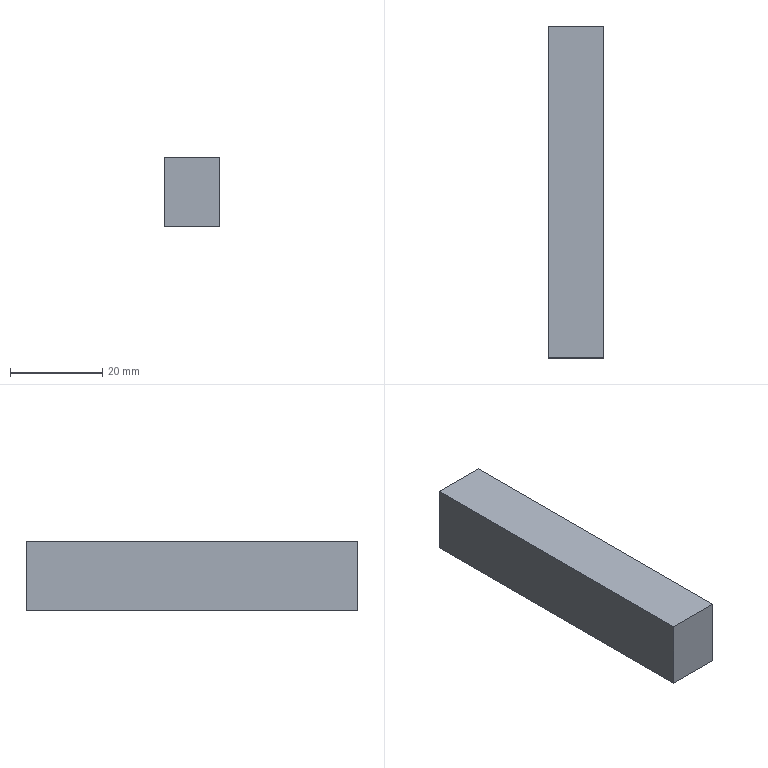Part | NX | features solid 2 | 1 solid | 6 faces | box 12 x 72 x 15 mm | volume 12960 mm3 | plane 6
STEP:
#1=CARTESIAN_POINT('',(546.,577.,-10.));
#2=VERTEX_POINT('',#1);
#3=CARTESIAN_POINT('',(558.,577.,-10.));
#4=VERTEX_POINT('',#3);
#5=CARTESIAN_POINT('',(582.,577.,-10.));
#6=DIRECTION('',(-1.,0.,0.));
#7=VECTOR('',#6,1000.);
#8=LINE('',#5,#7);
#9=EDGE_CURVE('',#2,#4,#8,.F.);
#10=ORIENTED_EDGE('',*,*,#9,.F.);
#11=CARTESIAN_POINT('',(546.,577.,-25.));
#12=VERTEX_POINT('',#11);
#13=CARTESIAN_POINT('',(546.,577.,84.523));
#14=DIRECTION('',(0.,0.,-1.));
#15=VECTOR('',#14,1000.);
#16=LINE('',#13,#15);
#17=EDGE_CURVE('',#2,#12,#16,.T.);
#18=ORIENTED_EDGE('',*,*,#17,.T.);
#19=CARTESIAN_POINT('',(558.,577.,-25.));
#20=VERTEX_POINT('',#19);
#21=CARTESIAN_POINT('',(525.,577.,-25.));
#22=DIRECTION('',(1.,0.,0.));
#23=VECTOR('',#22,1000.);
#24=LINE('',#21,#23);
#25=EDGE_CURVE('',#12,#20,#24,.T.);
#26=ORIENTED_EDGE('',*,*,#25,.T.);
#27=CARTESIAN_POINT('',(558.,577.,84.523));
#28=DIRECTION('',(0.,0.,-1.));
#29=VECTOR('',#28,1000.);
#30=LINE('',#27,#29);
#31=EDGE_CURVE('',#4,#20,#30,.T.);
#32=ORIENTED_EDGE('',*,*,#31,.F.);
#33=EDGE_LOOP('',(#10,#18,#26,#32));
#34=FACE_BOUND('',#33,.T.);
#35=CARTESIAN_POINT('',(546.,577.,-10.));
#36=DIRECTION('',(0.,-1.,0.));
#37=DIRECTION('',(0.,0.,-1.));
#38=AXIS2_PLACEMENT_3D('',#35,#36,#37);
#39=PLANE('',#38);
#40=ADVANCED_FACE('',(#34),#39,.T.);
#41=CARTESIAN_POINT('',(546.,649.,-10.));
#42=VERTEX_POINT('',#41);
#43=CARTESIAN_POINT('',(546.,649.,-25.));
#44=VERTEX_POINT('',#43);
#45=CARTESIAN_POINT('',(546.,649.,84.523));
#46=DIRECTION('',(0.,0.,-1.));
#47=VECTOR('',#46,1000.);
#48=LINE('',#45,#47);
#49=EDGE_CURVE('',#42,#44,#48,.T.);
#50=ORIENTED_EDGE('',*,*,#49,.F.);
#51=CARTESIAN_POINT('',(558.,649.,-10.));
#52=VERTEX_POINT('',#51);
#53=CARTESIAN_POINT('',(525.,649.,-10.));
#54=DIRECTION('',(1.,0.,0.));
#55=VECTOR('',#54,1000.);
#56=LINE('',#53,#55);
#57=EDGE_CURVE('',#42,#52,#56,.T.);
#58=ORIENTED_EDGE('',*,*,#57,.T.);
#59=CARTESIAN_POINT('',(558.,649.,-25.));
#60=VERTEX_POINT('',#59);
#61=CARTESIAN_POINT('',(558.,649.,84.523));
#62=DIRECTION('',(0.,0.,-1.));
#63=VECTOR('',#62,1000.);
#64=LINE('',#61,#63);
#65=EDGE_CURVE('',#52,#60,#64,.T.);
#66=ORIENTED_EDGE('',*,*,#65,.T.);
#67=CARTESIAN_POINT('',(525.,649.,-25.));
#68=DIRECTION('',(1.,0.,0.));
#69=VECTOR('',#68,1000.);
#70=LINE('',#67,#69);
#71=EDGE_CURVE('',#44,#60,#70,.T.);
#72=ORIENTED_EDGE('',*,*,#71,.F.);
#73=EDGE_LOOP('',(#50,#58,#66,#72));
#74=FACE_BOUND('',#73,.T.);
#75=CARTESIAN_POINT('',(546.,649.,-10.));
#76=DIRECTION('',(0.,-1.,0.));
#77=DIRECTION('',(0.,0.,-1.));
#78=AXIS2_PLACEMENT_3D('',#75,#76,#77);
#79=PLANE('',#78);
#80=ADVANCED_FACE('',(#74),#79,.F.);
#81=ORIENTED_EDGE('',*,*,#25,.F.);
#82=CARTESIAN_POINT('',(546.,669.,-25.));
#83=DIRECTION('',(0.,1.,0.));
#84=VECTOR('',#83,1000.);
#85=LINE('',#82,#84);
#86=EDGE_CURVE('',#12,#44,#85,.T.);
#87=ORIENTED_EDGE('',*,*,#86,.T.);
#88=ORIENTED_EDGE('',*,*,#71,.T.);
#89=CARTESIAN_POINT('',(558.,669.,-25.));
#90=DIRECTION('',(0.,1.,0.));
#91=VECTOR('',#90,1000.);
#92=LINE('',#89,#91);
#93=EDGE_CURVE('',#20,#60,#92,.T.);
#94=ORIENTED_EDGE('',*,*,#93,.F.);
#95=EDGE_LOOP('',(#81,#87,#88,#94));
#96=FACE_BOUND('',#95,.T.);
#97=CARTESIAN_POINT('',(525.,602.,-25.));
#98=DIRECTION('',(0.,0.,1.));
#99=DIRECTION('',(1.,0.,0.));
#100=AXIS2_PLACEMENT_3D('',#97,#98,#99);
#101=PLANE('',#100);
#102=ADVANCED_FACE('',(#96),#101,.F.);
#103=ORIENTED_EDGE('',*,*,#57,.F.);
#104=CARTESIAN_POINT('',(546.,669.,-10.));
#105=DIRECTION('',(0.,-1.,0.));
#106=VECTOR('',#105,1000.);
#107=LINE('',#104,#106);
#108=EDGE_CURVE('',#42,#2,#107,.T.);
#109=ORIENTED_EDGE('',*,*,#108,.T.);
#110=ORIENTED_EDGE('',*,*,#9,.T.);
#111=CARTESIAN_POINT('',(558.,692.,-10.));
#112=DIRECTION('',(0.,1.,0.));
#113=VECTOR('',#112,1000.);
#114=LINE('',#111,#113);
#115=EDGE_CURVE('',#4,#52,#114,.T.);
#116=ORIENTED_EDGE('',*,*,#115,.T.);
#117=EDGE_LOOP('',(#103,#109,#110,#116));
#118=FACE_BOUND('',#117,.T.);
#119=CARTESIAN_POINT('',(525.,602.,-10.));
#120=DIRECTION('',(0.,0.,1.));
#121=DIRECTION('',(1.,0.,0.));
#122=AXIS2_PLACEMENT_3D('',#119,#120,#121);
#123=PLANE('',#122);
#124=ADVANCED_FACE('',(#118),#123,.T.);
#125=ORIENTED_EDGE('',*,*,#17,.F.);
#126=ORIENTED_EDGE('',*,*,#108,.F.);
#127=ORIENTED_EDGE('',*,*,#49,.T.);
#128=ORIENTED_EDGE('',*,*,#86,.F.);
#129=EDGE_LOOP('',(#125,#126,#127,#128));
#130=FACE_BOUND('',#129,.T.);
#131=CARTESIAN_POINT('',(546.,669.,84.523));
#132=DIRECTION('',(1.,0.,0.));
#133=DIRECTION('',(0.,-1.,0.));
#134=AXIS2_PLACEMENT_3D('',#131,#132,#133);
#135=PLANE('',#134);
#136=ADVANCED_FACE('',(#130),#135,.F.);
#137=ORIENTED_EDGE('',*,*,#115,.F.);
#138=ORIENTED_EDGE('',*,*,#31,.T.);
#139=ORIENTED_EDGE('',*,*,#93,.T.);
#140=ORIENTED_EDGE('',*,*,#65,.F.);
#141=EDGE_LOOP('',(#137,#138,#139,#140));
#142=FACE_BOUND('',#141,.T.);
#143=CARTESIAN_POINT('',(558.,669.,84.523));
#144=DIRECTION('',(1.,0.,0.));
#145=DIRECTION('',(0.,-1.,0.));
#146=AXIS2_PLACEMENT_3D('',#143,#144,#145);
#147=PLANE('',#146);
#148=ADVANCED_FACE('',(#142),#147,.T.);
#149=CLOSED_SHELL('',(#40,#80,#102,#124,#136,#148));
#150=MANIFOLD_SOLID_BREP('',#149);
#151=(LENGTH_UNIT()NAMED_UNIT(*)SI_UNIT(.MILLI.,.METRE.));
#152=UNCERTAINTY_MEASURE_WITH_UNIT(LENGTH_MEASURE(0.00001),#151,'','');
#153=(NAMED_UNIT(*)PLANE_ANGLE_UNIT()SI_UNIT($,.RADIAN.));
#154=(NAMED_UNIT(*)SI_UNIT($,.STERADIAN.)SOLID_ANGLE_UNIT());
#155=(GEOMETRIC_REPRESENTATION_CONTEXT(3)GLOBAL_UNCERTAINTY_ASSIGNED_CONTEXT((#152))GLOBAL_UNIT_ASSIGNED_CONTEXT((#151,#153,#154))REPRESENTATION_CONTEXT('',''));
#156=ADVANCED_BREP_SHAPE_REPRESENTATION('',(#150),#155);